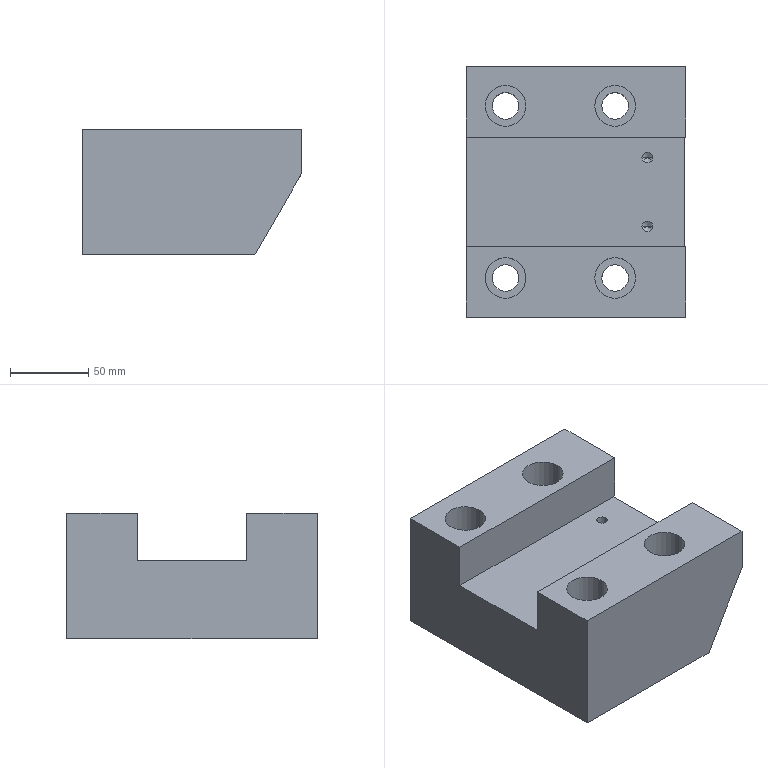Part | 1 solid | 45 faces | box 140 x 160 x 80 mm | volume 1213741 mm3 | cylinder 22 | plane 19 | cone 4 | commonest cylinder face diameters 17 x8 26 x8 6.8 x4 35.02 x2